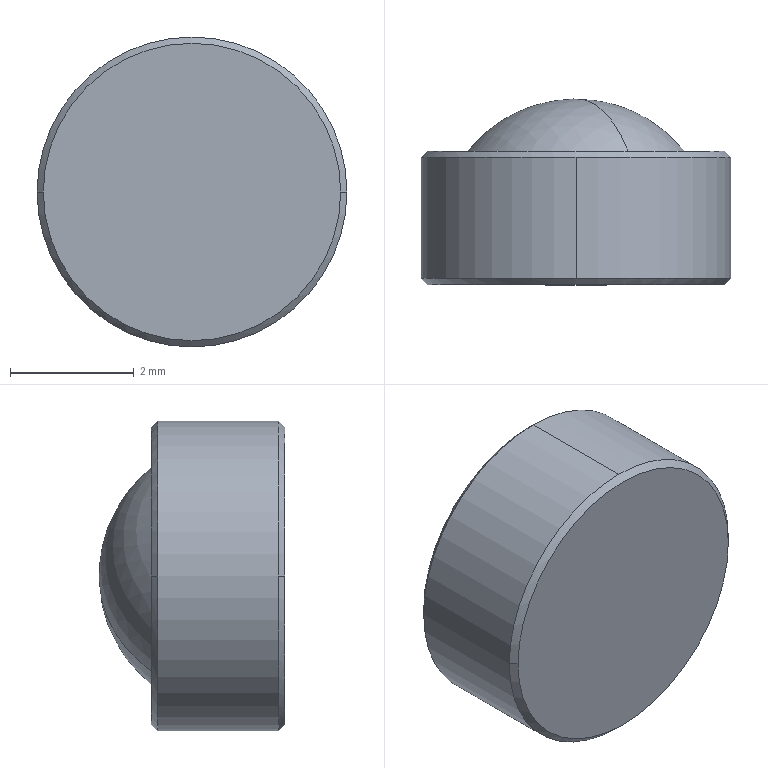Part | SolidWorks | features BaseBody 1 | 1 solid | 10 faces | box 5 x 3 x 5 mm | volume 46.543 mm3 | cone 4 | cylinder 2 | sphere 2 | plane 2 | commonest cylinder face diameters 5 x2
STEP:
#1=CARTESIAN_POINT('',(0.1,2.154,0.));
#2=VERTEX_POINT('',#1);
#3=CARTESIAN_POINT('',(4.9,2.154,0.));
#4=VERTEX_POINT('',#3);
#5=CARTESIAN_POINT('',(2.5,2.154,0.));
#6=DIRECTION('',(0.,1.,0.));
#7=DIRECTION('',(-1.,0.,0.));
#8=AXIS2_PLACEMENT_3D('',#5,#6,#7);
#9=CIRCLE('',#8,2.4);
#10=EDGE_CURVE('',#2,#4,#9,.T.);
#11=ORIENTED_EDGE('',*,*,#10,.F.);
#12=CARTESIAN_POINT('',(0.,2.054,0.));
#13=VERTEX_POINT('',#12);
#14=CARTESIAN_POINT('',(0.05,2.104,0.));
#15=DIRECTION('',(-0.7071,-0.7071,0.));
#16=VECTOR('',#15,1000.);
#17=LINE('',#14,#16);
#18=EDGE_CURVE('',#2,#13,#17,.T.);
#19=ORIENTED_EDGE('',*,*,#18,.T.);
#20=CARTESIAN_POINT('',(2.5,2.054,2.5));
#21=VERTEX_POINT('',#20);
#22=CARTESIAN_POINT('',(2.5,2.054,0.));
#23=DIRECTION('',(0.,1.,0.));
#24=DIRECTION('',(0.8776,0.,-0.4794));
#25=AXIS2_PLACEMENT_3D('',#22,#23,#24);
#26=CIRCLE('',#25,2.5);
#27=EDGE_CURVE('',#13,#21,#26,.T.);
#28=ORIENTED_EDGE('',*,*,#27,.T.);
#29=CARTESIAN_POINT('',(5.,2.054,0.));
#30=VERTEX_POINT('',#29);
#31=CARTESIAN_POINT('',(2.5,2.054,0.));
#32=DIRECTION('',(0.,1.,0.));
#33=DIRECTION('',(0.8776,0.,-0.4794));
#34=AXIS2_PLACEMENT_3D('',#31,#32,#33);
#35=CIRCLE('',#34,2.5);
#36=EDGE_CURVE('',#21,#30,#35,.T.);
#37=ORIENTED_EDGE('',*,*,#36,.T.);
#38=CARTESIAN_POINT('',(4.95,2.104,0.));
#39=DIRECTION('',(0.7071,-0.7071,0.));
#40=VECTOR('',#39,1000.);
#41=LINE('',#38,#40);
#42=EDGE_CURVE('',#4,#30,#41,.T.);
#43=ORIENTED_EDGE('',*,*,#42,.F.);
#44=EDGE_LOOP('',(#11,#19,#28,#37,#43));
#45=FACE_OUTER_BOUND('',#44,.T.);
#46=CARTESIAN_POINT('',(2.5,2.104,0.));
#47=DIRECTION('',(0.,-1.,0.));
#48=DIRECTION('',(1.,0.,0.));
#49=AXIS2_PLACEMENT_3D('',#46,#47,#48);
#50=CONICAL_SURFACE('',#49,2.45,0.7854);
#51=ADVANCED_FACE('',(#45),#50,.T.);
#52=CARTESIAN_POINT('',(2.5,0.1,-2.5));
#53=VERTEX_POINT('',#52);
#54=CARTESIAN_POINT('',(5.,0.1,0.));
#55=VERTEX_POINT('',#54);
#56=CARTESIAN_POINT('',(2.5,0.1,0.));
#57=DIRECTION('',(0.,-1.,0.));
#58=DIRECTION('',(1.,0.,0.));
#59=AXIS2_PLACEMENT_3D('',#56,#57,#58);
#60=CIRCLE('',#59,2.5);
#61=EDGE_CURVE('',#53,#55,#60,.T.);
#62=ORIENTED_EDGE('',*,*,#61,.F.);
#63=CARTESIAN_POINT('',(2.5,2.054,-2.5));
#64=VERTEX_POINT('',#63);
#65=CARTESIAN_POINT('',(2.5,1.5,-2.5));
#66=DIRECTION('',(0.,1.,0.));
#67=VECTOR('',#66,1000.);
#68=LINE('',#65,#67);
#69=EDGE_CURVE('',#53,#64,#68,.T.);
#70=ORIENTED_EDGE('',*,*,#69,.T.);
#71=CARTESIAN_POINT('',(2.5,2.054,0.));
#72=DIRECTION('',(0.,1.,0.));
#73=DIRECTION('',(0.8776,0.,-0.4794));
#74=AXIS2_PLACEMENT_3D('',#71,#72,#73);
#75=CIRCLE('',#74,2.5);
#76=EDGE_CURVE('',#30,#64,#75,.T.);
#77=ORIENTED_EDGE('',*,*,#76,.F.);
#78=ORIENTED_EDGE('',*,*,#36,.F.);
#79=CARTESIAN_POINT('',(2.5,0.1,2.5));
#80=VERTEX_POINT('',#79);
#81=CARTESIAN_POINT('',(2.5,1.5,2.5));
#82=DIRECTION('',(0.,1.,0.));
#83=VECTOR('',#82,1000.);
#84=LINE('',#81,#83);
#85=EDGE_CURVE('',#80,#21,#84,.T.);
#86=ORIENTED_EDGE('',*,*,#85,.F.);
#87=CARTESIAN_POINT('',(2.5,0.1,0.));
#88=DIRECTION('',(0.,-1.,0.));
#89=DIRECTION('',(1.,0.,0.));
#90=AXIS2_PLACEMENT_3D('',#87,#88,#89);
#91=CIRCLE('',#90,2.5);
#92=EDGE_CURVE('',#55,#80,#91,.T.);
#93=ORIENTED_EDGE('',*,*,#92,.F.);
#94=EDGE_LOOP('',(#62,#70,#77,#78,#86,#93));
#95=FACE_OUTER_BOUND('',#94,.T.);
#96=CARTESIAN_POINT('',(2.5,1.5,0.));
#97=DIRECTION('',(0.,1.,0.));
#98=DIRECTION('',(0.,0.,1.));
#99=AXIS2_PLACEMENT_3D('',#96,#97,#98);
#100=CYLINDRICAL_SURFACE('',#99,2.5);
#101=ADVANCED_FACE('',(#95),#100,.T.);
#102=CARTESIAN_POINT('',(4.9,0.,0.));
#103=VERTEX_POINT('',#102);
#104=CARTESIAN_POINT('',(0.1,0.,0.));
#105=VERTEX_POINT('',#104);
#106=CARTESIAN_POINT('',(2.5,0.,0.));
#107=DIRECTION('',(0.,-1.,0.));
#108=DIRECTION('',(-1.,0.,0.));
#109=AXIS2_PLACEMENT_3D('',#106,#107,#108);
#110=CIRCLE('',#109,2.4);
#111=EDGE_CURVE('',#103,#105,#110,.T.);
#112=ORIENTED_EDGE('',*,*,#111,.F.);
#113=CARTESIAN_POINT('',(4.95,0.05,0.));
#114=DIRECTION('',(0.7071,0.7071,0.));
#115=VECTOR('',#114,1000.);
#116=LINE('',#113,#115);
#117=EDGE_CURVE('',#103,#55,#116,.T.);
#118=ORIENTED_EDGE('',*,*,#117,.T.);
#119=ORIENTED_EDGE('',*,*,#92,.T.);
#120=CARTESIAN_POINT('',(0.,0.1,0.));
#121=VERTEX_POINT('',#120);
#122=CARTESIAN_POINT('',(2.5,0.1,0.));
#123=DIRECTION('',(0.,-1.,0.));
#124=DIRECTION('',(1.,0.,0.));
#125=AXIS2_PLACEMENT_3D('',#122,#123,#124);
#126=CIRCLE('',#125,2.5);
#127=EDGE_CURVE('',#80,#121,#126,.T.);
#128=ORIENTED_EDGE('',*,*,#127,.T.);
#129=CARTESIAN_POINT('',(0.05,0.05,0.));
#130=DIRECTION('',(-0.7071,0.7071,0.));
#131=VECTOR('',#130,1000.);
#132=LINE('',#129,#131);
#133=EDGE_CURVE('',#105,#121,#132,.T.);
#134=ORIENTED_EDGE('',*,*,#133,.F.);
#135=EDGE_LOOP('',(#112,#118,#119,#128,#134));
#136=FACE_OUTER_BOUND('',#135,.T.);
#137=CARTESIAN_POINT('',(2.5,0.05,0.));
#138=DIRECTION('',(0.,1.,0.));
#139=DIRECTION('',(-1.,0.,0.));
#140=AXIS2_PLACEMENT_3D('',#137,#138,#139);
#141=CONICAL_SURFACE('',#140,2.45,0.7854);
#142=ADVANCED_FACE('',(#136),#141,.T.);
#143=CARTESIAN_POINT('',(1.843,2.532,-1.203));
#144=VERTEX_POINT('',#143);
#145=CARTESIAN_POINT('',(3.341,2.154,1.539));
#146=VERTEX_POINT('',#145);
#147=CARTESIAN_POINT('',(2.5,0.7592,0.));
#148=DIRECTION('',(0.8776,0.,-0.4794));
#149=DIRECTION('',(-0.4794,0.,-0.8776));
#150=AXIS2_PLACEMENT_3D('',#147,#148,#149);
#151=CIRCLE('',#150,2.241);
#152=EDGE_CURVE('',#144,#146,#151,.T.);
#153=ORIENTED_EDGE('',*,*,#152,.F.);
#154=CARTESIAN_POINT('',(1.659,2.154,-1.539));
#155=VERTEX_POINT('',#154);
#156=CARTESIAN_POINT('',(2.5,0.7592,0.));
#157=DIRECTION('',(-0.8776,0.,0.4794));
#158=DIRECTION('',(0.4794,0.,0.8776));
#159=AXIS2_PLACEMENT_3D('',#156,#157,#158);
#160=CIRCLE('',#159,2.241);
#161=EDGE_CURVE('',#144,#155,#160,.T.);
#162=ORIENTED_EDGE('',*,*,#161,.T.);
#163=CARTESIAN_POINT('',(2.5,2.154,0.));
#164=DIRECTION('',(0.,1.,0.));
#165=DIRECTION('',(-0.8776,0.,0.4794));
#166=AXIS2_PLACEMENT_3D('',#163,#164,#165);
#167=CIRCLE('',#166,1.754);
#168=EDGE_CURVE('',#155,#146,#167,.T.);
#169=ORIENTED_EDGE('',*,*,#168,.T.);
#170=EDGE_LOOP('',(#153,#162,#169));
#171=FACE_OUTER_BOUND('',#170,.T.);
#172=CARTESIAN_POINT('',(2.5,0.7592,0.));
#173=DIRECTION('',(-0.8776,0.,0.4794));
#174=DIRECTION('',(0.3793,0.6115,0.6944));
#175=AXIS2_PLACEMENT_3D('',#172,#173,#174);
#176=SPHERICAL_SURFACE('',#175,2.241);
#177=ADVANCED_FACE('',(#171),#176,.T.);
#178=ORIENTED_EDGE('',*,*,#161,.F.);
#179=ORIENTED_EDGE('',*,*,#152,.T.);
#180=CARTESIAN_POINT('',(2.5,2.154,0.));
#181=DIRECTION('',(0.,1.,0.));
#182=DIRECTION('',(-0.8776,0.,0.4794));
#183=AXIS2_PLACEMENT_3D('',#180,#181,#182);
#184=CIRCLE('',#183,1.754);
#185=EDGE_CURVE('',#146,#155,#184,.T.);
#186=ORIENTED_EDGE('',*,*,#185,.T.);
#187=EDGE_LOOP('',(#178,#179,#186));
#188=FACE_OUTER_BOUND('',#187,.T.);
#189=CARTESIAN_POINT('',(2.5,0.7592,0.));
#190=DIRECTION('',(-0.8776,0.,0.4794));
#191=DIRECTION('',(0.3793,0.6115,0.6944));
#192=AXIS2_PLACEMENT_3D('',#189,#190,#191);
#193=SPHERICAL_SURFACE('',#192,2.241);
#194=ADVANCED_FACE('',(#188),#193,.T.);
#195=CARTESIAN_POINT('',(2.5,0.,0.));
#196=DIRECTION('',(0.,-1.,0.));
#197=DIRECTION('',(-1.,0.,0.));
#198=AXIS2_PLACEMENT_3D('',#195,#196,#197);
#199=CIRCLE('',#198,2.4);
#200=EDGE_CURVE('',#105,#103,#199,.T.);
#201=ORIENTED_EDGE('',*,*,#200,.T.);
#202=ORIENTED_EDGE('',*,*,#111,.T.);
#203=EDGE_LOOP('',(#201,#202));
#204=FACE_OUTER_BOUND('',#203,.T.);
#205=CARTESIAN_POINT('',(2.5,0.,0.));
#206=DIRECTION('',(0.,1.,0.));
#207=DIRECTION('',(1.,0.,0.));
#208=AXIS2_PLACEMENT_3D('',#205,#206,#207);
#209=PLANE('',#208);
#210=ADVANCED_FACE('',(#204),#209,.F.);
#211=ORIENTED_EDGE('',*,*,#117,.F.);
#212=ORIENTED_EDGE('',*,*,#200,.F.);
#213=ORIENTED_EDGE('',*,*,#133,.T.);
#214=CARTESIAN_POINT('',(2.5,0.1,0.));
#215=DIRECTION('',(0.,-1.,0.));
#216=DIRECTION('',(1.,0.,0.));
#217=AXIS2_PLACEMENT_3D('',#214,#215,#216);
#218=CIRCLE('',#217,2.5);
#219=EDGE_CURVE('',#121,#53,#218,.T.);
#220=ORIENTED_EDGE('',*,*,#219,.T.);
#221=ORIENTED_EDGE('',*,*,#61,.T.);
#222=EDGE_LOOP('',(#211,#212,#213,#220,#221));
#223=FACE_OUTER_BOUND('',#222,.T.);
#224=CARTESIAN_POINT('',(2.5,0.05,0.));
#225=DIRECTION('',(0.,1.,0.));
#226=DIRECTION('',(-1.,0.,0.));
#227=AXIS2_PLACEMENT_3D('',#224,#225,#226);
#228=CONICAL_SURFACE('',#227,2.45,0.7854);
#229=ADVANCED_FACE('',(#223),#228,.T.);
#230=ORIENTED_EDGE('',*,*,#69,.F.);
#231=ORIENTED_EDGE('',*,*,#219,.F.);
#232=ORIENTED_EDGE('',*,*,#127,.F.);
#233=ORIENTED_EDGE('',*,*,#85,.T.);
#234=ORIENTED_EDGE('',*,*,#27,.F.);
#235=CARTESIAN_POINT('',(2.5,2.054,0.));
#236=DIRECTION('',(0.,1.,0.));
#237=DIRECTION('',(0.8776,0.,-0.4794));
#238=AXIS2_PLACEMENT_3D('',#235,#236,#237);
#239=CIRCLE('',#238,2.5);
#240=EDGE_CURVE('',#64,#13,#239,.T.);
#241=ORIENTED_EDGE('',*,*,#240,.F.);
#242=EDGE_LOOP('',(#230,#231,#232,#233,#234,#241));
#243=FACE_OUTER_BOUND('',#242,.T.);
#244=CARTESIAN_POINT('',(2.5,1.5,0.));
#245=DIRECTION('',(0.,1.,0.));
#246=DIRECTION('',(0.,0.,1.));
#247=AXIS2_PLACEMENT_3D('',#244,#245,#246);
#248=CYLINDRICAL_SURFACE('',#247,2.5);
#249=ADVANCED_FACE('',(#243),#248,.T.);
#250=ORIENTED_EDGE('',*,*,#18,.F.);
#251=CARTESIAN_POINT('',(2.5,2.154,0.));
#252=DIRECTION('',(0.,1.,0.));
#253=DIRECTION('',(-1.,0.,0.));
#254=AXIS2_PLACEMENT_3D('',#251,#252,#253);
#255=CIRCLE('',#254,2.4);
#256=EDGE_CURVE('',#4,#2,#255,.T.);
#257=ORIENTED_EDGE('',*,*,#256,.F.);
#258=ORIENTED_EDGE('',*,*,#42,.T.);
#259=ORIENTED_EDGE('',*,*,#76,.T.);
#260=ORIENTED_EDGE('',*,*,#240,.T.);
#261=EDGE_LOOP('',(#250,#257,#258,#259,#260));
#262=FACE_OUTER_BOUND('',#261,.T.);
#263=CARTESIAN_POINT('',(2.5,2.104,0.));
#264=DIRECTION('',(0.,-1.,0.));
#265=DIRECTION('',(1.,0.,0.));
#266=AXIS2_PLACEMENT_3D('',#263,#264,#265);
#267=CONICAL_SURFACE('',#266,2.45,0.7854);
#268=ADVANCED_FACE('',(#262),#267,.T.);
#269=ORIENTED_EDGE('',*,*,#185,.F.);
#270=ORIENTED_EDGE('',*,*,#168,.F.);
#271=EDGE_LOOP('',(#269,#270));
#272=FACE_BOUND('',#271,.T.);
#273=ORIENTED_EDGE('',*,*,#256,.T.);
#274=ORIENTED_EDGE('',*,*,#10,.T.);
#275=EDGE_LOOP('',(#273,#274));
#276=FACE_OUTER_BOUND('',#275,.T.);
#277=CARTESIAN_POINT('',(0.,2.154,0.));
#278=DIRECTION('',(0.,1.,0.));
#279=DIRECTION('',(1.,0.,0.));
#280=AXIS2_PLACEMENT_3D('',#277,#278,#279);
#281=PLANE('',#280);
#282=ADVANCED_FACE('',(#272,#276),#281,.T.);
#283=CLOSED_SHELL('',(#51,#101,#142,#177,#194,#210,#229,#249,#268,#282));
#284=MANIFOLD_SOLID_BREP('',#283);
#285=CARTESIAN_POINT('',(0.,0.,0.));
#286=DIRECTION('',(0.,0.,1.));
#287=DIRECTION('',(1.,0.,0.));
#288=AXIS2_PLACEMENT_3D('',#285,#286,#287);
#289=(LENGTH_UNIT()NAMED_UNIT(*)SI_UNIT(.MILLI.,.METRE.));
#290=UNCERTAINTY_MEASURE_WITH_UNIT(LENGTH_MEASURE(0.00001),#289,'','');
#291=(NAMED_UNIT(*)PLANE_ANGLE_UNIT()SI_UNIT($,.RADIAN.));
#292=(NAMED_UNIT(*)SI_UNIT($,.STERADIAN.)SOLID_ANGLE_UNIT());
#293=(GEOMETRIC_REPRESENTATION_CONTEXT(3)GLOBAL_UNCERTAINTY_ASSIGNED_CONTEXT((#290))GLOBAL_UNIT_ASSIGNED_CONTEXT((#289,#291,#292))REPRESENTATION_CONTEXT('',''));
#294=ADVANCED_BREP_SHAPE_REPRESENTATION('',(#284,#288),#293);